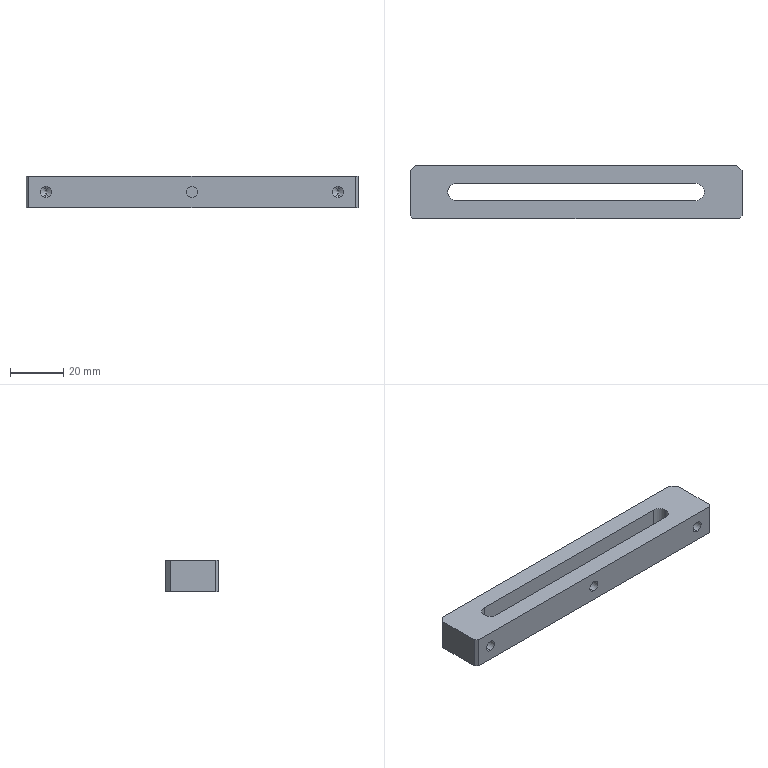Part | SolidWorks | features Chamfer 2, Extrusion 1, HoleWzd 1, ICE 1 | 1 solid | 25 faces | box 125 x 20 x 12 mm | volume 22020 mm3 | plane 12 | cylinder 9 | cone 4 | commonest cylinder face diameters 4.2 x6 6.6 x3
STEP:
#1=CARTESIAN_POINT('',(-55.,0.,8.1));
#2=VERTEX_POINT('',#1);
#3=CARTESIAN_POINT('',(-55.,0.,3.9));
#4=VERTEX_POINT('',#3);
#5=CARTESIAN_POINT('',(-55.,0.,6.));
#6=DIRECTION('',(0.,-1.,0.));
#7=DIRECTION('',(0.,0.,-1.));
#8=AXIS2_PLACEMENT_3D('',#5,#6,#7);
#9=CIRCLE('',#8,2.1);
#10=EDGE_CURVE('',#2,#4,#9,.T.);
#11=ORIENTED_EDGE('',*,*,#10,.F.);
#12=CARTESIAN_POINT('',(-55.,-10.,8.1));
#13=VERTEX_POINT('',#12);
#14=CARTESIAN_POINT('',(-55.,-10.,8.1));
#15=DIRECTION('',(0.,-1.,0.));
#16=VECTOR('',#15,1000.);
#17=LINE('',#14,#16);
#18=EDGE_CURVE('',#2,#13,#17,.T.);
#19=ORIENTED_EDGE('',*,*,#18,.T.);
#20=CARTESIAN_POINT('',(-55.,-10.,3.9));
#21=VERTEX_POINT('',#20);
#22=CARTESIAN_POINT('',(-55.,-10.,6.));
#23=DIRECTION('',(0.,-1.,0.));
#24=DIRECTION('',(0.,0.,-1.));
#25=AXIS2_PLACEMENT_3D('',#22,#23,#24);
#26=CIRCLE('',#25,2.1);
#27=EDGE_CURVE('',#13,#21,#26,.T.);
#28=ORIENTED_EDGE('',*,*,#27,.T.);
#29=CARTESIAN_POINT('',(-55.,-10.,3.9));
#30=DIRECTION('',(0.,-1.,0.));
#31=VECTOR('',#30,1000.);
#32=LINE('',#29,#31);
#33=EDGE_CURVE('',#4,#21,#32,.T.);
#34=ORIENTED_EDGE('',*,*,#33,.F.);
#35=EDGE_LOOP('',(#11,#19,#28,#34));
#36=FACE_OUTER_BOUND('',#35,.T.);
#37=CARTESIAN_POINT('',(-55.,-10.,6.));
#38=DIRECTION('',(0.,-1.,0.));
#39=DIRECTION('',(0.,0.,-1.));
#40=AXIS2_PLACEMENT_3D('',#37,#38,#39);
#41=CYLINDRICAL_SURFACE('',#40,2.1);
#42=ADVANCED_FACE('',(#36),#41,.F.);
#43=CARTESIAN_POINT('',(-55.,1.262,6.));
#44=VERTEX_POINT('',#43);
#45=CARTESIAN_POINT('',(-55.,0.,3.9));
#46=DIRECTION('',(0.,-0.515,-0.8572));
#47=VECTOR('',#46,1000.);
#48=LINE('',#45,#47);
#49=EDGE_CURVE('',#44,#4,#48,.T.);
#50=ORIENTED_EDGE('',*,*,#49,.F.);
#51=CARTESIAN_POINT('',(-55.,0.,8.1));
#52=DIRECTION('',(0.,-0.515,0.8572));
#53=VECTOR('',#52,1000.);
#54=LINE('',#51,#53);
#55=EDGE_CURVE('',#44,#2,#54,.T.);
#56=ORIENTED_EDGE('',*,*,#55,.T.);
#57=ORIENTED_EDGE('',*,*,#10,.T.);
#58=EDGE_LOOP('',(#50,#56,#57));
#59=FACE_OUTER_BOUND('',#58,.T.);
#60=CARTESIAN_POINT('',(-55.,0.,6.));
#61=DIRECTION('',(0.,-1.,0.));
#62=DIRECTION('',(0.,0.,-1.));
#63=AXIS2_PLACEMENT_3D('',#60,#61,#62);
#64=CONICAL_SURFACE('',#63,2.1,1.03);
#65=ADVANCED_FACE('',(#59),#64,.F.);
#66=CARTESIAN_POINT('',(0.,-3.3,8.1));
#67=VERTEX_POINT('',#66);
#68=CARTESIAN_POINT('',(0.,-3.3,3.9));
#69=VERTEX_POINT('',#68);
#70=CARTESIAN_POINT('',(0.,-3.3,6.));
#71=DIRECTION('',(0.,-1.,0.));
#72=DIRECTION('',(0.,0.,-1.));
#73=AXIS2_PLACEMENT_3D('',#70,#71,#72);
#74=CIRCLE('',#73,2.1);
#75=EDGE_CURVE('',#67,#69,#74,.T.);
#76=ORIENTED_EDGE('',*,*,#75,.F.);
#77=CARTESIAN_POINT('',(0.,-10.,8.1));
#78=VERTEX_POINT('',#77);
#79=CARTESIAN_POINT('',(0.,-10.,8.1));
#80=DIRECTION('',(0.,-1.,0.));
#81=VECTOR('',#80,1000.);
#82=LINE('',#79,#81);
#83=EDGE_CURVE('',#67,#78,#82,.T.);
#84=ORIENTED_EDGE('',*,*,#83,.T.);
#85=CARTESIAN_POINT('',(0.,-10.,3.9));
#86=VERTEX_POINT('',#85);
#87=CARTESIAN_POINT('',(0.,-10.,6.));
#88=DIRECTION('',(0.,-1.,0.));
#89=DIRECTION('',(0.,0.,-1.));
#90=AXIS2_PLACEMENT_3D('',#87,#88,#89);
#91=CIRCLE('',#90,2.1);
#92=EDGE_CURVE('',#78,#86,#91,.T.);
#93=ORIENTED_EDGE('',*,*,#92,.T.);
#94=CARTESIAN_POINT('',(0.,-10.,3.9));
#95=DIRECTION('',(0.,-1.,0.));
#96=VECTOR('',#95,1000.);
#97=LINE('',#94,#96);
#98=EDGE_CURVE('',#69,#86,#97,.T.);
#99=ORIENTED_EDGE('',*,*,#98,.F.);
#100=EDGE_LOOP('',(#76,#84,#93,#99));
#101=FACE_OUTER_BOUND('',#100,.T.);
#102=CARTESIAN_POINT('',(0.,-10.,6.));
#103=DIRECTION('',(0.,-1.,0.));
#104=DIRECTION('',(0.,0.,-1.));
#105=AXIS2_PLACEMENT_3D('',#102,#103,#104);
#106=CYLINDRICAL_SURFACE('',#105,2.1);
#107=ADVANCED_FACE('',(#101),#106,.F.);
#108=CARTESIAN_POINT('',(55.,0.,8.1));
#109=VERTEX_POINT('',#108);
#110=CARTESIAN_POINT('',(55.,0.,3.9));
#111=VERTEX_POINT('',#110);
#112=CARTESIAN_POINT('',(55.,0.,6.));
#113=DIRECTION('',(0.,-1.,0.));
#114=DIRECTION('',(0.,0.,-1.));
#115=AXIS2_PLACEMENT_3D('',#112,#113,#114);
#116=CIRCLE('',#115,2.1);
#117=EDGE_CURVE('',#109,#111,#116,.T.);
#118=ORIENTED_EDGE('',*,*,#117,.F.);
#119=CARTESIAN_POINT('',(55.,-10.,8.1));
#120=VERTEX_POINT('',#119);
#121=CARTESIAN_POINT('',(55.,-10.,8.1));
#122=DIRECTION('',(0.,-1.,0.));
#123=VECTOR('',#122,1000.);
#124=LINE('',#121,#123);
#125=EDGE_CURVE('',#109,#120,#124,.T.);
#126=ORIENTED_EDGE('',*,*,#125,.T.);
#127=CARTESIAN_POINT('',(55.,-10.,3.9));
#128=VERTEX_POINT('',#127);
#129=CARTESIAN_POINT('',(55.,-10.,6.));
#130=DIRECTION('',(0.,-1.,0.));
#131=DIRECTION('',(0.,0.,-1.));
#132=AXIS2_PLACEMENT_3D('',#129,#130,#131);
#133=CIRCLE('',#132,2.1);
#134=EDGE_CURVE('',#120,#128,#133,.T.);
#135=ORIENTED_EDGE('',*,*,#134,.T.);
#136=CARTESIAN_POINT('',(55.,-10.,3.9));
#137=DIRECTION('',(0.,-1.,0.));
#138=VECTOR('',#137,1000.);
#139=LINE('',#136,#138);
#140=EDGE_CURVE('',#111,#128,#139,.T.);
#141=ORIENTED_EDGE('',*,*,#140,.F.);
#142=EDGE_LOOP('',(#118,#126,#135,#141));
#143=FACE_OUTER_BOUND('',#142,.T.);
#144=CARTESIAN_POINT('',(55.,-10.,6.));
#145=DIRECTION('',(0.,-1.,0.));
#146=DIRECTION('',(0.,0.,-1.));
#147=AXIS2_PLACEMENT_3D('',#144,#145,#146);
#148=CYLINDRICAL_SURFACE('',#147,2.1);
#149=ADVANCED_FACE('',(#143),#148,.F.);
#150=CARTESIAN_POINT('',(55.,1.262,6.));
#151=VERTEX_POINT('',#150);
#152=CARTESIAN_POINT('',(55.,0.,3.9));
#153=DIRECTION('',(0.,-0.515,-0.8572));
#154=VECTOR('',#153,1000.);
#155=LINE('',#152,#154);
#156=EDGE_CURVE('',#151,#111,#155,.T.);
#157=ORIENTED_EDGE('',*,*,#156,.F.);
#158=CARTESIAN_POINT('',(55.,0.,8.1));
#159=DIRECTION('',(0.,-0.515,0.8572));
#160=VECTOR('',#159,1000.);
#161=LINE('',#158,#160);
#162=EDGE_CURVE('',#151,#109,#161,.T.);
#163=ORIENTED_EDGE('',*,*,#162,.T.);
#164=ORIENTED_EDGE('',*,*,#117,.T.);
#165=EDGE_LOOP('',(#157,#163,#164));
#166=FACE_OUTER_BOUND('',#165,.T.);
#167=CARTESIAN_POINT('',(55.,0.,6.));
#168=DIRECTION('',(0.,-1.,0.));
#169=DIRECTION('',(0.,0.,-1.));
#170=AXIS2_PLACEMENT_3D('',#167,#168,#169);
#171=CONICAL_SURFACE('',#170,2.1,1.03);
#172=ADVANCED_FACE('',(#166),#171,.F.);
#173=CARTESIAN_POINT('',(48.3,0.,0.));
#174=VERTEX_POINT('',#173);
#175=CARTESIAN_POINT('',(45.,3.3,0.));
#176=VERTEX_POINT('',#175);
#177=CARTESIAN_POINT('',(45.,0.,0.));
#178=DIRECTION('',(0.,0.,1.));
#179=DIRECTION('',(1.,0.,0.));
#180=AXIS2_PLACEMENT_3D('',#177,#178,#179);
#181=CIRCLE('',#180,3.3);
#182=EDGE_CURVE('',#174,#176,#181,.T.);
#183=ORIENTED_EDGE('',*,*,#182,.F.);
#184=CARTESIAN_POINT('',(48.3,0.,12.));
#185=VERTEX_POINT('',#184);
#186=CARTESIAN_POINT('',(48.3,0.,0.));
#187=DIRECTION('',(0.,0.,1.));
#188=VECTOR('',#187,1000.);
#189=LINE('',#186,#188);
#190=EDGE_CURVE('',#174,#185,#189,.T.);
#191=ORIENTED_EDGE('',*,*,#190,.T.);
#192=CARTESIAN_POINT('',(45.,3.3,12.));
#193=VERTEX_POINT('',#192);
#194=CARTESIAN_POINT('',(45.,0.,12.));
#195=DIRECTION('',(0.,0.,1.));
#196=DIRECTION('',(1.,0.,0.));
#197=AXIS2_PLACEMENT_3D('',#194,#195,#196);
#198=CIRCLE('',#197,3.3);
#199=EDGE_CURVE('',#185,#193,#198,.T.);
#200=ORIENTED_EDGE('',*,*,#199,.T.);
#201=CARTESIAN_POINT('',(45.,3.3,0.));
#202=DIRECTION('',(0.,0.,1.));
#203=VECTOR('',#202,1000.);
#204=LINE('',#201,#203);
#205=EDGE_CURVE('',#176,#193,#204,.T.);
#206=ORIENTED_EDGE('',*,*,#205,.F.);
#207=EDGE_LOOP('',(#183,#191,#200,#206));
#208=FACE_OUTER_BOUND('',#207,.T.);
#209=CARTESIAN_POINT('',(45.,0.,0.));
#210=DIRECTION('',(0.,0.,1.));
#211=DIRECTION('',(1.,0.,0.));
#212=AXIS2_PLACEMENT_3D('',#209,#210,#211);
#213=CYLINDRICAL_SURFACE('',#212,3.3);
#214=ADVANCED_FACE('',(#208),#213,.F.);
#215=CARTESIAN_POINT('',(62.5,-9.,12.));
#216=VERTEX_POINT('',#215);
#217=CARTESIAN_POINT('',(62.5,8.,12.));
#218=VERTEX_POINT('',#217);
#219=CARTESIAN_POINT('',(62.5,-10.,12.));
#220=DIRECTION('',(0.,1.,0.));
#221=VECTOR('',#220,1000.);
#222=LINE('',#219,#221);
#223=EDGE_CURVE('',#216,#218,#222,.T.);
#224=ORIENTED_EDGE('',*,*,#223,.F.);
#225=CARTESIAN_POINT('',(62.5,-9.,0.));
#226=VERTEX_POINT('',#225);
#227=CARTESIAN_POINT('',(62.5,-9.,12.));
#228=DIRECTION('',(0.,0.,-1.));
#229=VECTOR('',#228,1000.);
#230=LINE('',#227,#229);
#231=EDGE_CURVE('',#216,#226,#230,.T.);
#232=ORIENTED_EDGE('',*,*,#231,.T.);
#233=CARTESIAN_POINT('',(62.5,8.,0.));
#234=VERTEX_POINT('',#233);
#235=CARTESIAN_POINT('',(62.5,-10.,0.));
#236=DIRECTION('',(0.,1.,0.));
#237=VECTOR('',#236,1000.);
#238=LINE('',#235,#237);
#239=EDGE_CURVE('',#226,#234,#238,.T.);
#240=ORIENTED_EDGE('',*,*,#239,.T.);
#241=CARTESIAN_POINT('',(62.5,8.,12.));
#242=DIRECTION('',(0.,0.,1.));
#243=VECTOR('',#242,1000.);
#244=LINE('',#241,#243);
#245=EDGE_CURVE('',#234,#218,#244,.T.);
#246=ORIENTED_EDGE('',*,*,#245,.T.);
#247=EDGE_LOOP('',(#224,#232,#240,#246));
#248=FACE_OUTER_BOUND('',#247,.T.);
#249=CARTESIAN_POINT('',(62.5,-10.,12.));
#250=DIRECTION('',(-1.,0.,0.));
#251=DIRECTION('',(0.,0.,1.));
#252=AXIS2_PLACEMENT_3D('',#249,#250,#251);
#253=PLANE('',#252);
#254=ADVANCED_FACE('',(#248),#253,.F.);
#255=CARTESIAN_POINT('',(60.5,10.,0.));
#256=VERTEX_POINT('',#255);
#257=CARTESIAN_POINT('',(-60.5,10.,0.));
#258=VERTEX_POINT('',#257);
#259=CARTESIAN_POINT('',(-62.5,10.,0.));
#260=DIRECTION('',(-1.,0.,0.));
#261=VECTOR('',#260,1000.);
#262=LINE('',#259,#261);
#263=EDGE_CURVE('',#256,#258,#262,.T.);
#264=ORIENTED_EDGE('',*,*,#263,.T.);
#265=CARTESIAN_POINT('',(-60.5,10.,12.));
#266=VERTEX_POINT('',#265);
#267=CARTESIAN_POINT('',(-60.5,10.,12.));
#268=DIRECTION('',(0.,0.,1.));
#269=VECTOR('',#268,1000.);
#270=LINE('',#267,#269);
#271=EDGE_CURVE('',#258,#266,#270,.T.);
#272=ORIENTED_EDGE('',*,*,#271,.T.);
#273=CARTESIAN_POINT('',(60.5,10.,12.));
#274=VERTEX_POINT('',#273);
#275=CARTESIAN_POINT('',(-62.5,10.,12.));
#276=DIRECTION('',(-1.,0.,0.));
#277=VECTOR('',#276,1000.);
#278=LINE('',#275,#277);
#279=EDGE_CURVE('',#274,#266,#278,.T.);
#280=ORIENTED_EDGE('',*,*,#279,.F.);
#281=CARTESIAN_POINT('',(60.5,10.,12.));
#282=DIRECTION('',(0.,0.,-1.));
#283=VECTOR('',#282,1000.);
#284=LINE('',#281,#283);
#285=EDGE_CURVE('',#274,#256,#284,.T.);
#286=ORIENTED_EDGE('',*,*,#285,.T.);
#287=EDGE_LOOP('',(#264,#272,#280,#286));
#288=FACE_OUTER_BOUND('',#287,.T.);
#289=CARTESIAN_POINT('',(-62.5,10.,12.));
#290=DIRECTION('',(0.,-1.,0.));
#291=DIRECTION('',(0.,0.,-1.));
#292=AXIS2_PLACEMENT_3D('',#289,#290,#291);
#293=PLANE('',#292);
#294=ADVANCED_FACE('',(#288),#293,.F.);
#295=CARTESIAN_POINT('',(-62.5,8.,0.));
#296=VERTEX_POINT('',#295);
#297=CARTESIAN_POINT('',(-62.5,-9.,0.));
#298=VERTEX_POINT('',#297);
#299=CARTESIAN_POINT('',(-62.5,-10.,0.));
#300=DIRECTION('',(0.,-1.,0.));
#301=VECTOR('',#300,1000.);
#302=LINE('',#299,#301);
#303=EDGE_CURVE('',#296,#298,#302,.T.);
#304=ORIENTED_EDGE('',*,*,#303,.T.);
#305=CARTESIAN_POINT('',(-62.5,-9.,12.));
#306=VERTEX_POINT('',#305);
#307=CARTESIAN_POINT('',(-62.5,-9.,12.));
#308=DIRECTION('',(0.,0.,1.));
#309=VECTOR('',#308,1000.);
#310=LINE('',#307,#309);
#311=EDGE_CURVE('',#298,#306,#310,.T.);
#312=ORIENTED_EDGE('',*,*,#311,.T.);
#313=CARTESIAN_POINT('',(-62.5,8.,12.));
#314=VERTEX_POINT('',#313);
#315=CARTESIAN_POINT('',(-62.5,-10.,12.));
#316=DIRECTION('',(0.,-1.,0.));
#317=VECTOR('',#316,1000.);
#318=LINE('',#315,#317);
#319=EDGE_CURVE('',#314,#306,#318,.T.);
#320=ORIENTED_EDGE('',*,*,#319,.F.);
#321=CARTESIAN_POINT('',(-62.5,8.,12.));
#322=DIRECTION('',(0.,0.,-1.));
#323=VECTOR('',#322,1000.);
#324=LINE('',#321,#323);
#325=EDGE_CURVE('',#314,#296,#324,.T.);
#326=ORIENTED_EDGE('',*,*,#325,.T.);
#327=EDGE_LOOP('',(#304,#312,#320,#326));
#328=FACE_OUTER_BOUND('',#327,.T.);
#329=CARTESIAN_POINT('',(-62.5,-10.,12.));
#330=DIRECTION('',(1.,0.,0.));
#331=DIRECTION('',(0.,0.,-1.));
#332=AXIS2_PLACEMENT_3D('',#329,#330,#331);
#333=PLANE('',#332);
#334=ADVANCED_FACE('',(#328),#333,.F.);
#335=CARTESIAN_POINT('',(-55.,-10.,6.));
#336=DIRECTION('',(0.,-1.,0.));
#337=DIRECTION('',(0.,0.,-1.));
#338=AXIS2_PLACEMENT_3D('',#335,#336,#337);
#339=CIRCLE('',#338,2.1);
#340=EDGE_CURVE('',#21,#13,#339,.T.);
#341=ORIENTED_EDGE('',*,*,#340,.F.);
#342=ORIENTED_EDGE('',*,*,#27,.F.);
#343=EDGE_LOOP('',(#341,#342));
#344=FACE_BOUND('',#343,.T.);
#345=CARTESIAN_POINT('',(0.,-10.,6.));
#346=DIRECTION('',(0.,-1.,0.));
#347=DIRECTION('',(0.,0.,-1.));
#348=AXIS2_PLACEMENT_3D('',#345,#346,#347);
#349=CIRCLE('',#348,2.1);
#350=EDGE_CURVE('',#86,#78,#349,.T.);
#351=ORIENTED_EDGE('',*,*,#350,.F.);
#352=ORIENTED_EDGE('',*,*,#92,.F.);
#353=EDGE_LOOP('',(#351,#352));
#354=FACE_BOUND('',#353,.T.);
#355=CARTESIAN_POINT('',(55.,-10.,6.));
#356=DIRECTION('',(0.,-1.,0.));
#357=DIRECTION('',(0.,0.,-1.));
#358=AXIS2_PLACEMENT_3D('',#355,#356,#357);
#359=CIRCLE('',#358,2.1);
#360=EDGE_CURVE('',#128,#120,#359,.T.);
#361=ORIENTED_EDGE('',*,*,#360,.F.);
#362=ORIENTED_EDGE('',*,*,#134,.F.);
#363=EDGE_LOOP('',(#361,#362));
#364=FACE_BOUND('',#363,.T.);
#365=CARTESIAN_POINT('',(-61.5,-10.,12.));
#366=VERTEX_POINT('',#365);
#367=CARTESIAN_POINT('',(61.5,-10.,12.));
#368=VERTEX_POINT('',#367);
#369=CARTESIAN_POINT('',(-62.5,-10.,12.));
#370=DIRECTION('',(1.,0.,0.));
#371=VECTOR('',#370,1000.);
#372=LINE('',#369,#371);
#373=EDGE_CURVE('',#366,#368,#372,.T.);
#374=ORIENTED_EDGE('',*,*,#373,.F.);
#375=CARTESIAN_POINT('',(-61.5,-10.,0.));
#376=VERTEX_POINT('',#375);
#377=CARTESIAN_POINT('',(-61.5,-10.,12.));
#378=DIRECTION('',(0.,0.,-1.));
#379=VECTOR('',#378,1000.);
#380=LINE('',#377,#379);
#381=EDGE_CURVE('',#366,#376,#380,.T.);
#382=ORIENTED_EDGE('',*,*,#381,.T.);
#383=CARTESIAN_POINT('',(61.5,-10.,0.));
#384=VERTEX_POINT('',#383);
#385=CARTESIAN_POINT('',(-62.5,-10.,0.));
#386=DIRECTION('',(1.,0.,0.));
#387=VECTOR('',#386,1000.);
#388=LINE('',#385,#387);
#389=EDGE_CURVE('',#376,#384,#388,.T.);
#390=ORIENTED_EDGE('',*,*,#389,.T.);
#391=CARTESIAN_POINT('',(61.5,-10.,12.));
#392=DIRECTION('',(0.,0.,1.));
#393=VECTOR('',#392,1000.);
#394=LINE('',#391,#393);
#395=EDGE_CURVE('',#384,#368,#394,.T.);
#396=ORIENTED_EDGE('',*,*,#395,.T.);
#397=EDGE_LOOP('',(#374,#382,#390,#396));
#398=FACE_OUTER_BOUND('',#397,.T.);
#399=CARTESIAN_POINT('',(-62.5,-10.,12.));
#400=DIRECTION('',(0.,1.,0.));
#401=DIRECTION('',(0.,0.,1.));
#402=AXIS2_PLACEMENT_3D('',#399,#400,#401);
#403=PLANE('',#402);
#404=ADVANCED_FACE('',(#344,#354,#364,#398),#403,.F.);
#405=CARTESIAN_POINT('',(-45.,-3.3,12.));
#406=VERTEX_POINT('',#405);
#407=CARTESIAN_POINT('',(45.,-3.3,12.));
#408=VERTEX_POINT('',#407);
#409=CARTESIAN_POINT('',(-45.,-3.3,12.));
#410=DIRECTION('',(1.,0.,0.));
#411=VECTOR('',#410,1000.);
#412=LINE('',#409,#411);
#413=EDGE_CURVE('',#406,#408,#412,.T.);
#414=ORIENTED_EDGE('',*,*,#413,.F.);
#415=CARTESIAN_POINT('',(-45.,3.3,12.));
#416=VERTEX_POINT('',#415);
#417=CARTESIAN_POINT('',(-45.,0.,12.));
#418=DIRECTION('',(0.,0.,1.));
#419=DIRECTION('',(1.,0.,0.));
#420=AXIS2_PLACEMENT_3D('',#417,#418,#419);
#421=CIRCLE('',#420,3.3);
#422=EDGE_CURVE('',#416,#406,#421,.T.);
#423=ORIENTED_EDGE('',*,*,#422,.F.);
#424=CARTESIAN_POINT('',(-45.,3.3,12.));
#425=DIRECTION('',(-1.,0.,0.));
#426=VECTOR('',#425,1000.);
#427=LINE('',#424,#426);
#428=EDGE_CURVE('',#193,#416,#427,.T.);
#429=ORIENTED_EDGE('',*,*,#428,.F.);
#430=ORIENTED_EDGE('',*,*,#199,.F.);
#431=CARTESIAN_POINT('',(45.,0.,12.));
#432=DIRECTION('',(0.,0.,1.));
#433=DIRECTION('',(1.,0.,0.));
#434=AXIS2_PLACEMENT_3D('',#431,#432,#433);
#435=CIRCLE('',#434,3.3);
#436=EDGE_CURVE('',#408,#185,#435,.T.);
#437=ORIENTED_EDGE('',*,*,#436,.F.);
#438=EDGE_LOOP('',(#414,#423,#429,#430,#437));
#439=FACE_BOUND('',#438,.T.);
#440=ORIENTED_EDGE('',*,*,#319,.T.);
#441=CARTESIAN_POINT('',(-61.5,-10.,12.));
#442=DIRECTION('',(0.7071,-0.7071,0.));
#443=VECTOR('',#442,1000.);
#444=LINE('',#441,#443);
#445=EDGE_CURVE('',#306,#366,#444,.T.);
#446=ORIENTED_EDGE('',*,*,#445,.T.);
#447=ORIENTED_EDGE('',*,*,#373,.T.);
#448=CARTESIAN_POINT('',(62.5,-9.,12.));
#449=DIRECTION('',(0.7071,0.7071,0.));
#450=VECTOR('',#449,1000.);
#451=LINE('',#448,#450);
#452=EDGE_CURVE('',#368,#216,#451,.T.);
#453=ORIENTED_EDGE('',*,*,#452,.T.);
#454=ORIENTED_EDGE('',*,*,#223,.T.);
#455=CARTESIAN_POINT('',(60.5,10.,12.));
#456=DIRECTION('',(-0.7071,0.7071,0.));
#457=VECTOR('',#456,1000.);
#458=LINE('',#455,#457);
#459=EDGE_CURVE('',#218,#274,#458,.T.);
#460=ORIENTED_EDGE('',*,*,#459,.T.);
#461=ORIENTED_EDGE('',*,*,#279,.T.);
#462=CARTESIAN_POINT('',(-62.5,8.,12.));
#463=DIRECTION('',(-0.7071,-0.7071,0.));
#464=VECTOR('',#463,1000.);
#465=LINE('',#462,#464);
#466=EDGE_CURVE('',#266,#314,#465,.T.);
#467=ORIENTED_EDGE('',*,*,#466,.T.);
#468=EDGE_LOOP('',(#440,#446,#447,#453,#454,#460,#461,#467));
#469=FACE_OUTER_BOUND('',#468,.T.);
#470=CARTESIAN_POINT('',(0.,0.,12.));
#471=DIRECTION('',(0.,0.,-1.));
#472=DIRECTION('',(-1.,0.,0.));
#473=AXIS2_PLACEMENT_3D('',#470,#471,#472);
#474=PLANE('',#473);
#475=ADVANCED_FACE('',(#439,#469),#474,.F.);
#476=CARTESIAN_POINT('',(-45.,3.3,0.));
#477=VERTEX_POINT('',#476);
#478=CARTESIAN_POINT('',(-45.,-3.3,0.));
#479=VERTEX_POINT('',#478);
#480=CARTESIAN_POINT('',(-45.,0.,0.));
#481=DIRECTION('',(0.,0.,1.));
#482=DIRECTION('',(1.,0.,0.));
#483=AXIS2_PLACEMENT_3D('',#480,#481,#482);
#484=CIRCLE('',#483,3.3);
#485=EDGE_CURVE('',#477,#479,#484,.T.);
#486=ORIENTED_EDGE('',*,*,#485,.T.);
#487=CARTESIAN_POINT('',(45.,-3.3,0.));
#488=VERTEX_POINT('',#487);
#489=CARTESIAN_POINT('',(-45.,-3.3,0.));
#490=DIRECTION('',(1.,0.,0.));
#491=VECTOR('',#490,1000.);
#492=LINE('',#489,#491);
#493=EDGE_CURVE('',#479,#488,#492,.T.);
#494=ORIENTED_EDGE('',*,*,#493,.T.);
#495=CARTESIAN_POINT('',(45.,0.,0.));
#496=DIRECTION('',(0.,0.,1.));
#497=DIRECTION('',(1.,0.,0.));
#498=AXIS2_PLACEMENT_3D('',#495,#496,#497);
#499=CIRCLE('',#498,3.3);
#500=EDGE_CURVE('',#488,#174,#499,.T.);
#501=ORIENTED_EDGE('',*,*,#500,.T.);
#502=ORIENTED_EDGE('',*,*,#182,.T.);
#503=CARTESIAN_POINT('',(-45.,3.3,0.));
#504=DIRECTION('',(-1.,0.,0.));
#505=VECTOR('',#504,1000.);
#506=LINE('',#503,#505);
#507=EDGE_CURVE('',#176,#477,#506,.T.);
#508=ORIENTED_EDGE('',*,*,#507,.T.);
#509=EDGE_LOOP('',(#486,#494,#501,#502,#508));
#510=FACE_BOUND('',#509,.T.);
#511=ORIENTED_EDGE('',*,*,#389,.F.);
#512=CARTESIAN_POINT('',(-35.75,-35.75,0.));
#513=DIRECTION('',(-0.7071,0.7071,0.));
#514=VECTOR('',#513,1000.);
#515=LINE('',#512,#514);
#516=EDGE_CURVE('',#376,#298,#515,.T.);
#517=ORIENTED_EDGE('',*,*,#516,.T.);
#518=ORIENTED_EDGE('',*,*,#303,.F.);
#519=CARTESIAN_POINT('',(-35.25,35.25,0.));
#520=DIRECTION('',(0.7071,0.7071,0.));
#521=VECTOR('',#520,1000.);
#522=LINE('',#519,#521);
#523=EDGE_CURVE('',#296,#258,#522,.T.);
#524=ORIENTED_EDGE('',*,*,#523,.T.);
#525=ORIENTED_EDGE('',*,*,#263,.F.);
#526=CARTESIAN_POINT('',(35.25,35.25,0.));
#527=DIRECTION('',(0.7071,-0.7071,0.));
#528=VECTOR('',#527,1000.);
#529=LINE('',#526,#528);
#530=EDGE_CURVE('',#256,#234,#529,.T.);
#531=ORIENTED_EDGE('',*,*,#530,.T.);
#532=ORIENTED_EDGE('',*,*,#239,.F.);
#533=CARTESIAN_POINT('',(35.75,-35.75,0.));
#534=DIRECTION('',(-0.7071,-0.7071,0.));
#535=VECTOR('',#534,1000.);
#536=LINE('',#533,#535);
#537=EDGE_CURVE('',#226,#384,#536,.T.);
#538=ORIENTED_EDGE('',*,*,#537,.T.);
#539=EDGE_LOOP('',(#511,#517,#518,#524,#525,#531,#532,#538));
#540=FACE_OUTER_BOUND('',#539,.T.);
#541=CARTESIAN_POINT('',(0.,0.,0.));
#542=DIRECTION('',(0.,0.,-1.));
#543=DIRECTION('',(-1.,0.,0.));
#544=AXIS2_PLACEMENT_3D('',#541,#542,#543);
#545=PLANE('',#544);
#546=ADVANCED_FACE('',(#510,#540),#545,.T.);
#547=ORIENTED_EDGE('',*,*,#422,.T.);
#548=CARTESIAN_POINT('',(-45.,-3.3,0.));
#549=DIRECTION('',(0.,0.,1.));
#550=VECTOR('',#549,1000.);
#551=LINE('',#548,#550);
#552=EDGE_CURVE('',#479,#406,#551,.T.);
#553=ORIENTED_EDGE('',*,*,#552,.F.);
#554=ORIENTED_EDGE('',*,*,#485,.F.);
#555=CARTESIAN_POINT('',(-45.,3.3,0.));
#556=DIRECTION('',(0.,0.,1.));
#557=VECTOR('',#556,1000.);
#558=LINE('',#555,#557);
#559=EDGE_CURVE('',#477,#416,#558,.T.);
#560=ORIENTED_EDGE('',*,*,#559,.T.);
#561=EDGE_LOOP('',(#547,#553,#554,#560));
#562=FACE_OUTER_BOUND('',#561,.T.);
#563=CARTESIAN_POINT('',(-45.,0.,0.));
#564=DIRECTION('',(0.,0.,1.));
#565=DIRECTION('',(1.,0.,0.));
#566=AXIS2_PLACEMENT_3D('',#563,#564,#565);
#567=CYLINDRICAL_SURFACE('',#566,3.3);
#568=ADVANCED_FACE('',(#562),#567,.F.);
#569=ORIENTED_EDGE('',*,*,#428,.T.);
#570=ORIENTED_EDGE('',*,*,#559,.F.);
#571=ORIENTED_EDGE('',*,*,#507,.F.);
#572=ORIENTED_EDGE('',*,*,#205,.T.);
#573=EDGE_LOOP('',(#569,#570,#571,#572));
#574=FACE_OUTER_BOUND('',#573,.T.);
#575=CARTESIAN_POINT('',(-45.,3.3,0.));
#576=DIRECTION('',(0.,1.,0.));
#577=DIRECTION('',(0.,0.,1.));
#578=AXIS2_PLACEMENT_3D('',#575,#576,#577);
#579=PLANE('',#578);
#580=ADVANCED_FACE('',(#574),#579,.F.);
#581=ORIENTED_EDGE('',*,*,#190,.F.);
#582=ORIENTED_EDGE('',*,*,#500,.F.);
#583=CARTESIAN_POINT('',(45.,-3.3,0.));
#584=DIRECTION('',(0.,0.,1.));
#585=VECTOR('',#584,1000.);
#586=LINE('',#583,#585);
#587=EDGE_CURVE('',#488,#408,#586,.T.);
#588=ORIENTED_EDGE('',*,*,#587,.T.);
#589=ORIENTED_EDGE('',*,*,#436,.T.);
#590=EDGE_LOOP('',(#581,#582,#588,#589));
#591=FACE_OUTER_BOUND('',#590,.T.);
#592=CARTESIAN_POINT('',(45.,0.,0.));
#593=DIRECTION('',(0.,0.,1.));
#594=DIRECTION('',(1.,0.,0.));
#595=AXIS2_PLACEMENT_3D('',#592,#593,#594);
#596=CYLINDRICAL_SURFACE('',#595,3.3);
#597=ADVANCED_FACE('',(#591),#596,.F.);
#598=CARTESIAN_POINT('',(0.,-3.3,6.));
#599=DIRECTION('',(0.,-1.,0.));
#600=DIRECTION('',(0.,0.,-1.));
#601=AXIS2_PLACEMENT_3D('',#598,#599,#600);
#602=CIRCLE('',#601,2.1);
#603=EDGE_CURVE('',#69,#67,#602,.T.);
#604=ORIENTED_EDGE('',*,*,#603,.T.);
#605=ORIENTED_EDGE('',*,*,#75,.T.);
#606=EDGE_LOOP('',(#604,#605));
#607=FACE_BOUND('',#606,.T.);
#608=ORIENTED_EDGE('',*,*,#413,.T.);
#609=ORIENTED_EDGE('',*,*,#587,.F.);
#610=ORIENTED_EDGE('',*,*,#493,.F.);
#611=ORIENTED_EDGE('',*,*,#552,.T.);
#612=EDGE_LOOP('',(#608,#609,#610,#611));
#613=FACE_OUTER_BOUND('',#612,.T.);
#614=CARTESIAN_POINT('',(-45.,-3.3,0.));
#615=DIRECTION('',(0.,-1.,0.));
#616=DIRECTION('',(0.,0.,-1.));
#617=AXIS2_PLACEMENT_3D('',#614,#615,#616);
#618=PLANE('',#617);
#619=ADVANCED_FACE('',(#607,#613),#618,.F.);
#620=ORIENTED_EDGE('',*,*,#162,.F.);
#621=ORIENTED_EDGE('',*,*,#156,.T.);
#622=CARTESIAN_POINT('',(55.,0.,6.));
#623=DIRECTION('',(0.,-1.,0.));
#624=DIRECTION('',(0.,0.,-1.));
#625=AXIS2_PLACEMENT_3D('',#622,#623,#624);
#626=CIRCLE('',#625,2.1);
#627=EDGE_CURVE('',#111,#109,#626,.T.);
#628=ORIENTED_EDGE('',*,*,#627,.T.);
#629=EDGE_LOOP('',(#620,#621,#628));
#630=FACE_OUTER_BOUND('',#629,.T.);
#631=CARTESIAN_POINT('',(55.,0.,6.));
#632=DIRECTION('',(0.,-1.,0.));
#633=DIRECTION('',(0.,0.,-1.));
#634=AXIS2_PLACEMENT_3D('',#631,#632,#633);
#635=CONICAL_SURFACE('',#634,2.1,1.03);
#636=ADVANCED_FACE('',(#630),#635,.F.);
#637=ORIENTED_EDGE('',*,*,#125,.F.);
#638=ORIENTED_EDGE('',*,*,#627,.F.);
#639=ORIENTED_EDGE('',*,*,#140,.T.);
#640=ORIENTED_EDGE('',*,*,#360,.T.);
#641=EDGE_LOOP('',(#637,#638,#639,#640));
#642=FACE_OUTER_BOUND('',#641,.T.);
#643=CARTESIAN_POINT('',(55.,-10.,6.));
#644=DIRECTION('',(0.,-1.,0.));
#645=DIRECTION('',(0.,0.,-1.));
#646=AXIS2_PLACEMENT_3D('',#643,#644,#645);
#647=CYLINDRICAL_SURFACE('',#646,2.1);
#648=ADVANCED_FACE('',(#642),#647,.F.);
#649=ORIENTED_EDGE('',*,*,#83,.F.);
#650=ORIENTED_EDGE('',*,*,#603,.F.);
#651=ORIENTED_EDGE('',*,*,#98,.T.);
#652=ORIENTED_EDGE('',*,*,#350,.T.);
#653=EDGE_LOOP('',(#649,#650,#651,#652));
#654=FACE_OUTER_BOUND('',#653,.T.);
#655=CARTESIAN_POINT('',(0.,-10.,6.));
#656=DIRECTION('',(0.,-1.,0.));
#657=DIRECTION('',(0.,0.,-1.));
#658=AXIS2_PLACEMENT_3D('',#655,#656,#657);
#659=CYLINDRICAL_SURFACE('',#658,2.1);
#660=ADVANCED_FACE('',(#654),#659,.F.);
#661=ORIENTED_EDGE('',*,*,#55,.F.);
#662=ORIENTED_EDGE('',*,*,#49,.T.);
#663=CARTESIAN_POINT('',(-55.,0.,6.));
#664=DIRECTION('',(0.,-1.,0.));
#665=DIRECTION('',(0.,0.,-1.));
#666=AXIS2_PLACEMENT_3D('',#663,#664,#665);
#667=CIRCLE('',#666,2.1);
#668=EDGE_CURVE('',#4,#2,#667,.T.);
#669=ORIENTED_EDGE('',*,*,#668,.T.);
#670=EDGE_LOOP('',(#661,#662,#669));
#671=FACE_OUTER_BOUND('',#670,.T.);
#672=CARTESIAN_POINT('',(-55.,0.,6.));
#673=DIRECTION('',(0.,-1.,0.));
#674=DIRECTION('',(0.,0.,-1.));
#675=AXIS2_PLACEMENT_3D('',#672,#673,#674);
#676=CONICAL_SURFACE('',#675,2.1,1.03);
#677=ADVANCED_FACE('',(#671),#676,.F.);
#678=ORIENTED_EDGE('',*,*,#18,.F.);
#679=ORIENTED_EDGE('',*,*,#668,.F.);
#680=ORIENTED_EDGE('',*,*,#33,.T.);
#681=ORIENTED_EDGE('',*,*,#340,.T.);
#682=EDGE_LOOP('',(#678,#679,#680,#681));
#683=FACE_OUTER_BOUND('',#682,.T.);
#684=CARTESIAN_POINT('',(-55.,-10.,6.));
#685=DIRECTION('',(0.,-1.,0.));
#686=DIRECTION('',(0.,0.,-1.));
#687=AXIS2_PLACEMENT_3D('',#684,#685,#686);
#688=CYLINDRICAL_SURFACE('',#687,2.1);
#689=ADVANCED_FACE('',(#683),#688,.F.);
#690=ORIENTED_EDGE('',*,*,#466,.F.);
#691=ORIENTED_EDGE('',*,*,#271,.F.);
#692=ORIENTED_EDGE('',*,*,#523,.F.);
#693=ORIENTED_EDGE('',*,*,#325,.F.);
#694=EDGE_LOOP('',(#690,#691,#692,#693));
#695=FACE_OUTER_BOUND('',#694,.T.);
#696=CARTESIAN_POINT('',(-62.5,8.,12.));
#697=DIRECTION('',(0.7071,-0.7071,0.));
#698=DIRECTION('',(0.,0.,-1.));
#699=AXIS2_PLACEMENT_3D('',#696,#697,#698);
#700=PLANE('',#699);
#701=ADVANCED_FACE('',(#695),#700,.F.);
#702=ORIENTED_EDGE('',*,*,#459,.F.);
#703=ORIENTED_EDGE('',*,*,#245,.F.);
#704=ORIENTED_EDGE('',*,*,#530,.F.);
#705=ORIENTED_EDGE('',*,*,#285,.F.);
#706=EDGE_LOOP('',(#702,#703,#704,#705));
#707=FACE_OUTER_BOUND('',#706,.T.);
#708=CARTESIAN_POINT('',(60.5,10.,12.));
#709=DIRECTION('',(-0.7071,-0.7071,0.));
#710=DIRECTION('',(0.,0.,-1.));
#711=AXIS2_PLACEMENT_3D('',#708,#709,#710);
#712=PLANE('',#711);
#713=ADVANCED_FACE('',(#707),#712,.F.);
#714=ORIENTED_EDGE('',*,*,#445,.F.);
#715=ORIENTED_EDGE('',*,*,#311,.F.);
#716=ORIENTED_EDGE('',*,*,#516,.F.);
#717=ORIENTED_EDGE('',*,*,#381,.F.);
#718=EDGE_LOOP('',(#714,#715,#716,#717));
#719=FACE_OUTER_BOUND('',#718,.T.);
#720=CARTESIAN_POINT('',(-61.5,-10.,12.));
#721=DIRECTION('',(0.7071,0.7071,0.));
#722=DIRECTION('',(0.,0.,-1.));
#723=AXIS2_PLACEMENT_3D('',#720,#721,#722);
#724=PLANE('',#723);
#725=ADVANCED_FACE('',(#719),#724,.F.);
#726=ORIENTED_EDGE('',*,*,#452,.F.);
#727=ORIENTED_EDGE('',*,*,#395,.F.);
#728=ORIENTED_EDGE('',*,*,#537,.F.);
#729=ORIENTED_EDGE('',*,*,#231,.F.);
#730=EDGE_LOOP('',(#726,#727,#728,#729));
#731=FACE_OUTER_BOUND('',#730,.T.);
#732=CARTESIAN_POINT('',(62.5,-9.,12.));
#733=DIRECTION('',(-0.7071,0.7071,0.));
#734=DIRECTION('',(0.,0.,-1.));
#735=AXIS2_PLACEMENT_3D('',#732,#733,#734);
#736=PLANE('',#735);
#737=ADVANCED_FACE('',(#731),#736,.F.);
#738=CLOSED_SHELL('',(#42,#65,#107,#149,#172,#214,#254,#294,#334,#404,#475,#546,#568,#580,#597,#619,#636,#648,#660,#677,#689,#701,#713,#725,#737));
#739=MANIFOLD_SOLID_BREP('',#738);
#740=CARTESIAN_POINT('',(0.,0.,0.));
#741=DIRECTION('',(0.,0.,1.));
#742=DIRECTION('',(1.,0.,0.));
#743=AXIS2_PLACEMENT_3D('',#740,#741,#742);
#744=(LENGTH_UNIT()NAMED_UNIT(*)SI_UNIT(.MILLI.,.METRE.));
#745=UNCERTAINTY_MEASURE_WITH_UNIT(LENGTH_MEASURE(0.00001),#744,'','');
#746=(NAMED_UNIT(*)PLANE_ANGLE_UNIT()SI_UNIT($,.RADIAN.));
#747=(NAMED_UNIT(*)SI_UNIT($,.STERADIAN.)SOLID_ANGLE_UNIT());
#748=(GEOMETRIC_REPRESENTATION_CONTEXT(3)GLOBAL_UNCERTAINTY_ASSIGNED_CONTEXT((#745))GLOBAL_UNIT_ASSIGNED_CONTEXT((#744,#746,#747))REPRESENTATION_CONTEXT('',''));
#749=ADVANCED_BREP_SHAPE_REPRESENTATION('',(#739,#743),#748);